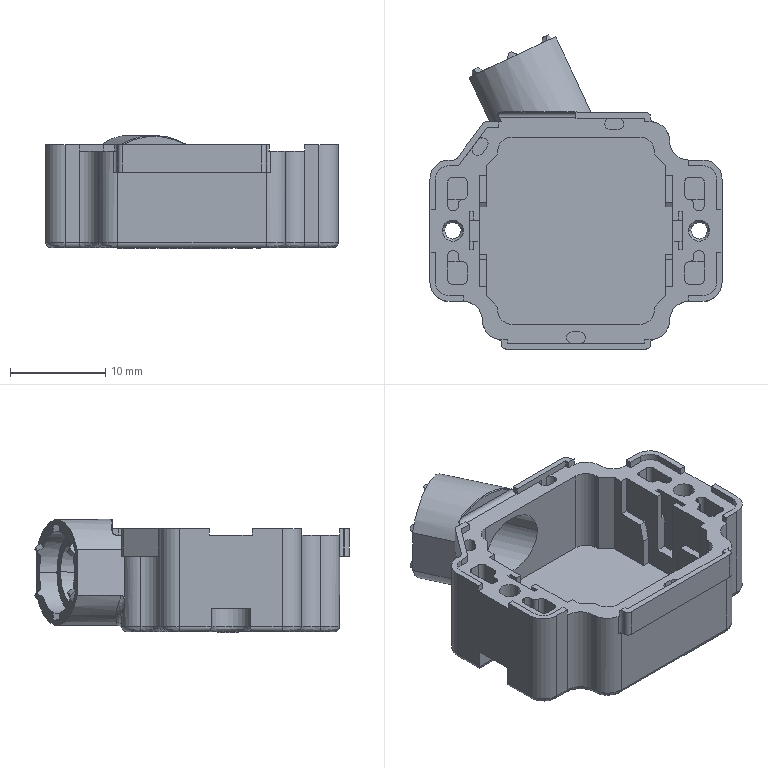Part | STEP file | 21E8-005-1072-P4_1_1_1_1 | 1 solid | 382 faces | box 30.6 x 32.912 x 11.855 mm | volume 2766 mm3 | plane 232 | cylinder 102 | spline 44 | cone 4 | commonest cylinder face diameters 1 x43 4 x12 1.2 x9 2.2 x8 10 x6 0.8 x4